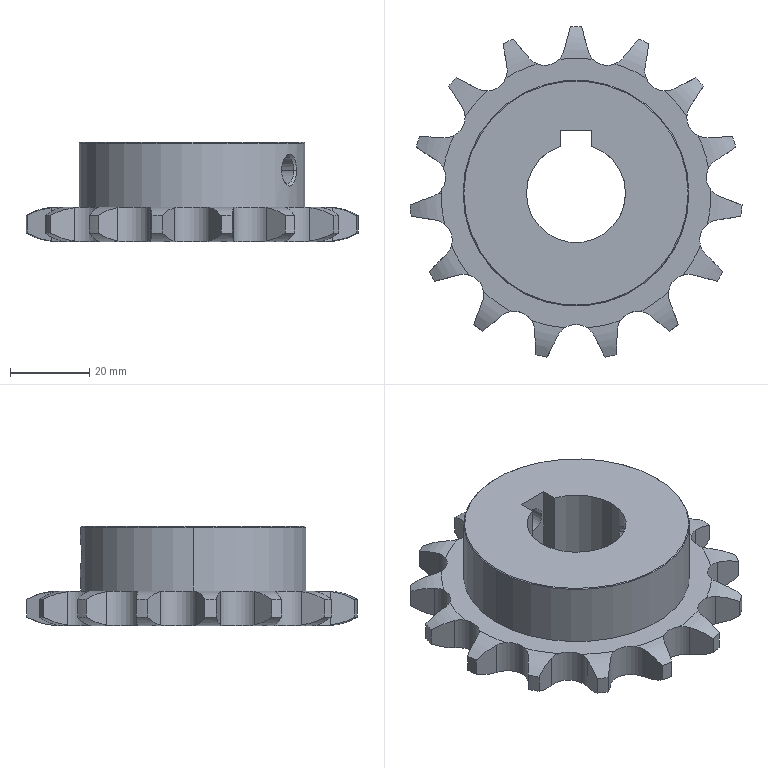Part | STEP file | _BSP50B15-N-25_B.stp | 1 solid | 118 faces | box 83.791 x 83.357 x 25 mm | volume 63531 mm3 | cylinder 44 | plane 36 | torus 32 | cone 6 | commonest cylinder face diameters 10.16 x20 84 x15 6.647 x4 25 x3 57 x2